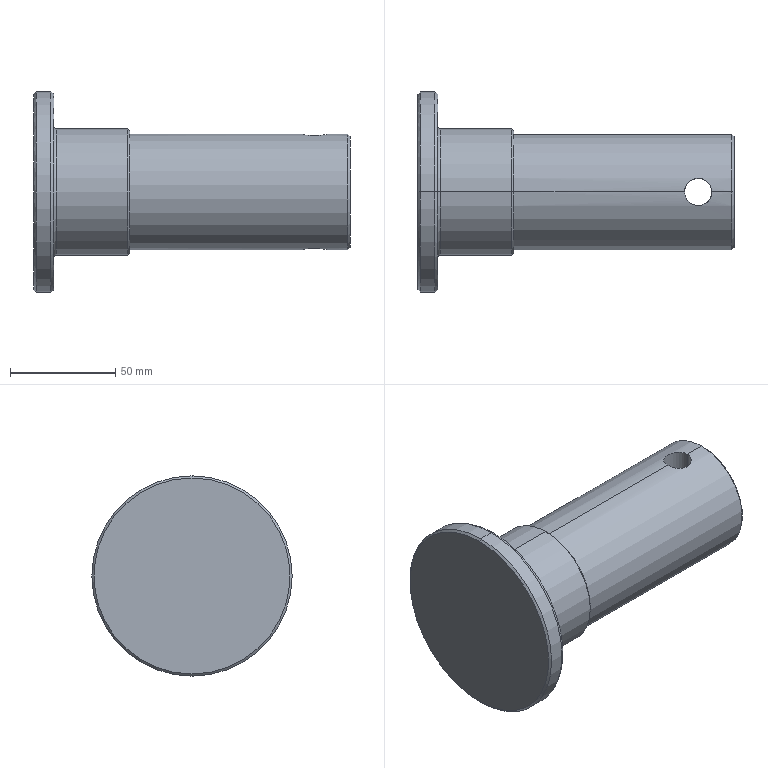Part | SolidWorks | features Chamfer 1, Fillet 1, ICE 1, Revolution 1 | 1 solid | 22 faces | box 150 x 95 x 95 mm | volume 409672 mm3 | cylinder 8 | cone 8 | plane 4 | torus 2 | commonest cylinder face diameters 13 x2 55 x2 60 x2 95 x2
STEP:
#1=CARTESIAN_POINT('',(126.5,0.,-27.5));
#2=VERTEX_POINT('',#1);
#3=CARTESIAN_POINT('',(139.5,0.,-27.5));
#4=VERTEX_POINT('',#3);
#5=CARTESIAN_POINT('',(126.5,0.,-27.5));
#6=CARTESIAN_POINT('',(126.5,-0.425,-27.5));
#7=CARTESIAN_POINT('',(126.541,-0.8485,-27.49));
#8=CARTESIAN_POINT('',(126.709,-1.692,-27.451));
#9=CARTESIAN_POINT('',(126.834,-2.099,-27.423));
#10=CARTESIAN_POINT('',(127.077,-2.687,-27.369));
#11=CARTESIAN_POINT('',(127.168,-2.878,-27.35));
#12=CARTESIAN_POINT('',(127.369,-3.254,-27.307));
#13=CARTESIAN_POINT('',(127.48,-3.439,-27.285));
#14=CARTESIAN_POINT('',(127.834,-3.968,-27.215));
#15=CARTESIAN_POINT('',(128.102,-4.294,-27.164));
#16=CARTESIAN_POINT('',(128.701,-4.894,-27.063));
#17=CARTESIAN_POINT('',(129.034,-5.167,-27.011));
#18=CARTESIAN_POINT('',(129.736,-5.637,-26.917));
#19=CARTESIAN_POINT('',(130.109,-5.837,-26.874));
#20=CARTESIAN_POINT('',(130.702,-6.084,-26.819));
#21=CARTESIAN_POINT('',(130.904,-6.156,-26.802));
#22=CARTESIAN_POINT('',(131.311,-6.28,-26.773));
#23=CARTESIAN_POINT('',(131.722,-6.384,-26.749));
#24=CARTESIAN_POINT('',(132.143,-6.447,-26.734));
#25=CARTESIAN_POINT('',(132.567,-6.489,-26.723));
#26=CARTESIAN_POINT('',(132.783,-6.5,-26.721));
#27=CARTESIAN_POINT('',(133.426,-6.5,-26.721));
#28=CARTESIAN_POINT('',(133.849,-6.458,-26.731));
#29=CARTESIAN_POINT('',(134.684,-6.293,-26.771));
#30=CARTESIAN_POINT('',(135.098,-6.167,-26.8));
#31=CARTESIAN_POINT('',(135.883,-5.841,-26.873));
#32=CARTESIAN_POINT('',(136.256,-5.642,-26.916));
#33=CARTESIAN_POINT('',(136.787,-5.287,-26.987));
#34=CARTESIAN_POINT('',(136.96,-5.159,-27.012));
#35=CARTESIAN_POINT('',(137.288,-4.89,-27.062));
#36=CARTESIAN_POINT('',(137.444,-4.748,-27.087));
#37=CARTESIAN_POINT('',(137.892,-4.301,-27.163));
#38=CARTESIAN_POINT('',(138.163,-3.972,-27.214));
#39=CARTESIAN_POINT('',(138.638,-3.263,-27.308));
#40=CARTESIAN_POINT('',(138.838,-2.89,-27.351));
#41=CARTESIAN_POINT('',(139.082,-2.303,-27.404));
#42=CARTESIAN_POINT('',(139.154,-2.103,-27.42));
#43=CARTESIAN_POINT('',(139.279,-1.693,-27.449));
#44=CARTESIAN_POINT('',(139.332,-1.484,-27.461));
#45=CARTESIAN_POINT('',(139.458,-0.8559,-27.49));
#46=CARTESIAN_POINT('',(139.5,-0.431,-27.5));
#47=CARTESIAN_POINT('',(139.5,0.,-27.5));
#48=B_SPLINE_CURVE_WITH_KNOTS('',3,(#5,#6,#7,#8,#9,#10,#11,#12,#13,#14,#15,#16,#17,#18,#19,#20,#21,#22,#23,#24,#25,#26,#27,#28,#29,#30,#31,#32,#33,#34,#35,#36,#37,#38,#39,#40,#41,#42,#43,#44,#45,#46,#47),.UNSPECIFIED.,.F.,.F.,(4,2,2,2,2,2,2,2,2,1,2,2,2,2,2,2,2,2,2,2,2,4),(0.02039,0.02167,0.02294,0.02358,0.02422,0.02549,0.02677,0.02804,0.02868,0.02931,0.02995,0.03059,0.03186,0.03314,0.03441,0.03505,0.03569,0.03696,0.03823,0.03887,0.03951,0.04078),.UNSPECIFIED.);
#49=EDGE_CURVE('',#2,#4,#48,.T.);
#50=ORIENTED_EDGE('',*,*,#49,.F.);
#51=CARTESIAN_POINT('',(126.5,0.,27.5));
#52=VERTEX_POINT('',#51);
#53=CARTESIAN_POINT('',(126.5,0.,-47.5));
#54=DIRECTION('',(0.,0.,1.));
#55=VECTOR('',#54,1000.);
#56=LINE('',#53,#55);
#57=EDGE_CURVE('',#2,#52,#56,.T.);
#58=ORIENTED_EDGE('',*,*,#57,.T.);
#59=CARTESIAN_POINT('',(139.5,0.,27.5));
#60=VERTEX_POINT('',#59);
#61=CARTESIAN_POINT('',(139.5,0.,27.5));
#62=CARTESIAN_POINT('',(139.5,-0.4311,27.5));
#63=CARTESIAN_POINT('',(139.458,-0.8547,27.49));
#64=CARTESIAN_POINT('',(139.333,-1.479,27.461));
#65=CARTESIAN_POINT('',(139.281,-1.686,27.449));
#66=CARTESIAN_POINT('',(139.157,-2.095,27.421));
#67=CARTESIAN_POINT('',(139.084,-2.298,27.405));
#68=CARTESIAN_POINT('',(138.839,-2.888,27.351));
#69=CARTESIAN_POINT('',(138.639,-3.261,27.308));
#70=CARTESIAN_POINT('',(138.285,-3.79,27.238));
#71=CARTESIAN_POINT('',(138.157,-3.962,27.214));
#72=CARTESIAN_POINT('',(137.887,-4.291,27.164));
#73=CARTESIAN_POINT('',(137.744,-4.448,27.138));
#74=CARTESIAN_POINT('',(137.296,-4.896,27.062));
#75=CARTESIAN_POINT('',(136.97,-5.165,27.012));
#76=CARTESIAN_POINT('',(136.26,-5.64,26.917));
#77=CARTESIAN_POINT('',(135.884,-5.841,26.873));
#78=CARTESIAN_POINT('',(135.298,-6.084,26.819));
#79=CARTESIAN_POINT('',(135.098,-6.156,26.802));
#80=CARTESIAN_POINT('',(134.69,-6.28,26.773));
#81=CARTESIAN_POINT('',(134.481,-6.333,26.761));
#82=CARTESIAN_POINT('',(133.851,-6.458,26.731));
#83=CARTESIAN_POINT('',(133.428,-6.5,26.721));
#84=CARTESIAN_POINT('',(132.577,-6.5,26.721));
#85=CARTESIAN_POINT('',(132.145,-6.458,26.731));
#86=CARTESIAN_POINT('',(131.31,-6.291,26.771));
#87=CARTESIAN_POINT('',(130.904,-6.167,26.8));
#88=CARTESIAN_POINT('',(130.312,-5.922,26.855));
#89=CARTESIAN_POINT('',(130.117,-5.83,26.875));
#90=CARTESIAN_POINT('',(129.743,-5.629,26.918));
#91=CARTESIAN_POINT('',(129.561,-5.52,26.941));
#92=CARTESIAN_POINT('',(129.21,-5.285,26.988));
#93=CARTESIAN_POINT('',(129.04,-5.159,27.012));
#94=CARTESIAN_POINT('',(128.712,-4.89,27.062));
#95=CARTESIAN_POINT('',(128.554,-4.746,27.088));
#96=CARTESIAN_POINT('',(128.102,-4.294,27.164));
#97=CARTESIAN_POINT('',(127.834,-3.967,27.215));
#98=CARTESIAN_POINT('',(127.363,-3.265,27.308));
#99=CARTESIAN_POINT('',(127.159,-2.884,27.351));
#100=CARTESIAN_POINT('',(126.833,-2.099,27.423));
#101=CARTESIAN_POINT('',(126.71,-1.693,27.451));
#102=CARTESIAN_POINT('',(126.584,-1.066,27.48));
#103=CARTESIAN_POINT('',(126.553,-0.8521,27.488));
#104=CARTESIAN_POINT('',(126.51,-0.4255,27.498));
#105=CARTESIAN_POINT('',(126.5,-0.2125,27.5));
#106=CARTESIAN_POINT('',(126.5,0.,27.5));
#107=B_SPLINE_CURVE_WITH_KNOTS('',3,(#61,#62,#63,#64,#65,#66,#67,#68,#69,#70,#71,#72,#73,#74,#75,#76,#77,#78,#79,#80,#81,#82,#83,#84,#85,#86,#87,#88,#89,#90,#91,#92,#93,#94,#95,#96,#97,#98,#99,#100,#101,#102,#103,#104,#105,#106),.UNSPECIFIED.,.F.,.F.,(4,2,2,2,2,2,2,2,2,2,2,2,2,2,2,2,2,2,2,2,2,2,4),(0.,0.001275,0.001912,0.002549,0.003824,0.004461,0.005099,0.006373,0.007648,0.008285,0.008923,0.0102,0.01147,0.01275,0.01338,0.01402,0.01466,0.0153,0.01657,0.01785,0.01912,0.01976,0.02039),.UNSPECIFIED.);
#108=EDGE_CURVE('',#60,#52,#107,.T.);
#109=ORIENTED_EDGE('',*,*,#108,.F.);
#110=CARTESIAN_POINT('',(139.5,0.,-47.5));
#111=DIRECTION('',(0.,0.,1.));
#112=VECTOR('',#111,1000.);
#113=LINE('',#110,#112);
#114=EDGE_CURVE('',#4,#60,#113,.T.);
#115=ORIENTED_EDGE('',*,*,#114,.F.);
#116=EDGE_LOOP('',(#50,#58,#109,#115));
#117=FACE_OUTER_BOUND('',#116,.T.);
#118=CARTESIAN_POINT('',(133.,0.,-47.5));
#119=DIRECTION('',(0.,0.,1.));
#120=DIRECTION('',(1.,0.,0.));
#121=AXIS2_PLACEMENT_3D('',#118,#119,#120);
#122=CYLINDRICAL_SURFACE('',#121,6.5);
#123=ADVANCED_FACE('',(#117),#122,.F.);
#124=CARTESIAN_POINT('',(150.,0.,-26.5));
#125=VERTEX_POINT('',#124);
#126=CARTESIAN_POINT('',(150.,0.,26.5));
#127=VERTEX_POINT('',#126);
#128=CARTESIAN_POINT('',(150.,0.,0.));
#129=DIRECTION('',(1.,0.,0.));
#130=DIRECTION('',(0.,0.,1.));
#131=AXIS2_PLACEMENT_3D('',#128,#129,#130);
#132=CIRCLE('',#131,26.5);
#133=EDGE_CURVE('',#125,#127,#132,.T.);
#134=ORIENTED_EDGE('',*,*,#133,.F.);
#135=CARTESIAN_POINT('',(149.,0.,-27.5));
#136=VERTEX_POINT('',#135);
#137=CARTESIAN_POINT('',(149.,0.,-27.5));
#138=DIRECTION('',(-0.7071,0.,-0.7071));
#139=VECTOR('',#138,1000.);
#140=LINE('',#137,#139);
#141=EDGE_CURVE('',#125,#136,#140,.T.);
#142=ORIENTED_EDGE('',*,*,#141,.T.);
#143=CARTESIAN_POINT('',(149.,0.,27.5));
#144=VERTEX_POINT('',#143);
#145=CARTESIAN_POINT('',(149.,0.,0.));
#146=DIRECTION('',(-1.,0.,0.));
#147=DIRECTION('',(0.,0.,1.));
#148=AXIS2_PLACEMENT_3D('',#145,#146,#147);
#149=CIRCLE('',#148,27.5);
#150=EDGE_CURVE('',#144,#136,#149,.T.);
#151=ORIENTED_EDGE('',*,*,#150,.F.);
#152=CARTESIAN_POINT('',(149.,0.,27.5));
#153=DIRECTION('',(-0.7071,0.,0.7071));
#154=VECTOR('',#153,1000.);
#155=LINE('',#152,#154);
#156=EDGE_CURVE('',#127,#144,#155,.T.);
#157=ORIENTED_EDGE('',*,*,#156,.F.);
#158=EDGE_LOOP('',(#134,#142,#151,#157));
#159=FACE_OUTER_BOUND('',#158,.T.);
#160=CARTESIAN_POINT('',(149.,0.,0.));
#161=DIRECTION('',(-1.,0.,0.));
#162=DIRECTION('',(0.,0.,1.));
#163=AXIS2_PLACEMENT_3D('',#160,#161,#162);
#164=CONICAL_SURFACE('',#163,27.5,0.7854);
#165=ADVANCED_FACE('',(#159),#164,.T.);
#166=CARTESIAN_POINT('',(45.5,0.,-29.));
#167=VERTEX_POINT('',#166);
#168=CARTESIAN_POINT('',(45.5,0.,29.));
#169=VERTEX_POINT('',#168);
#170=CARTESIAN_POINT('',(45.5,0.,0.));
#171=DIRECTION('',(1.,0.,0.));
#172=DIRECTION('',(0.,0.,1.));
#173=AXIS2_PLACEMENT_3D('',#170,#171,#172);
#174=CIRCLE('',#173,29.);
#175=EDGE_CURVE('',#167,#169,#174,.T.);
#176=ORIENTED_EDGE('',*,*,#175,.F.);
#177=CARTESIAN_POINT('',(44.5,0.,-30.));
#178=VERTEX_POINT('',#177);
#179=CARTESIAN_POINT('',(44.5,0.,-30.));
#180=DIRECTION('',(-0.7071,0.,-0.7071));
#181=VECTOR('',#180,1000.);
#182=LINE('',#179,#181);
#183=EDGE_CURVE('',#167,#178,#182,.T.);
#184=ORIENTED_EDGE('',*,*,#183,.T.);
#185=CARTESIAN_POINT('',(44.5,0.,30.));
#186=VERTEX_POINT('',#185);
#187=CARTESIAN_POINT('',(44.5,0.,0.));
#188=DIRECTION('',(-1.,0.,0.));
#189=DIRECTION('',(0.,0.,1.));
#190=AXIS2_PLACEMENT_3D('',#187,#188,#189);
#191=CIRCLE('',#190,30.);
#192=EDGE_CURVE('',#186,#178,#191,.T.);
#193=ORIENTED_EDGE('',*,*,#192,.F.);
#194=CARTESIAN_POINT('',(44.5,0.,30.));
#195=DIRECTION('',(-0.7071,0.,0.7071));
#196=VECTOR('',#195,1000.);
#197=LINE('',#194,#196);
#198=EDGE_CURVE('',#169,#186,#197,.T.);
#199=ORIENTED_EDGE('',*,*,#198,.F.);
#200=EDGE_LOOP('',(#176,#184,#193,#199));
#201=FACE_OUTER_BOUND('',#200,.T.);
#202=CARTESIAN_POINT('',(44.5,0.,0.));
#203=DIRECTION('',(-1.,0.,0.));
#204=DIRECTION('',(0.,0.,1.));
#205=AXIS2_PLACEMENT_3D('',#202,#203,#204);
#206=CONICAL_SURFACE('',#205,30.,0.7854);
#207=ADVANCED_FACE('',(#201),#206,.T.);
#208=CARTESIAN_POINT('',(0.,0.,46.5));
#209=VERTEX_POINT('',#208);
#210=CARTESIAN_POINT('',(0.,0.,-46.5));
#211=VERTEX_POINT('',#210);
#212=CARTESIAN_POINT('',(0.,0.,0.));
#213=DIRECTION('',(-1.,0.,0.));
#214=DIRECTION('',(0.,0.,-1.));
#215=AXIS2_PLACEMENT_3D('',#212,#213,#214);
#216=CIRCLE('',#215,46.5);
#217=EDGE_CURVE('',#209,#211,#216,.T.);
#218=ORIENTED_EDGE('',*,*,#217,.F.);
#219=CARTESIAN_POINT('',(1.,0.,47.5));
#220=VERTEX_POINT('',#219);
#221=CARTESIAN_POINT('',(0.,0.,46.5));
#222=DIRECTION('',(0.7071,0.,0.7071));
#223=VECTOR('',#222,1000.);
#224=LINE('',#221,#223);
#225=EDGE_CURVE('',#209,#220,#224,.T.);
#226=ORIENTED_EDGE('',*,*,#225,.T.);
#227=CARTESIAN_POINT('',(1.,0.,-47.5));
#228=VERTEX_POINT('',#227);
#229=CARTESIAN_POINT('',(1.,0.,0.));
#230=DIRECTION('',(1.,0.,0.));
#231=DIRECTION('',(0.,0.,-1.));
#232=AXIS2_PLACEMENT_3D('',#229,#230,#231);
#233=CIRCLE('',#232,47.5);
#234=EDGE_CURVE('',#228,#220,#233,.T.);
#235=ORIENTED_EDGE('',*,*,#234,.F.);
#236=CARTESIAN_POINT('',(0.,0.,-46.5));
#237=DIRECTION('',(0.7071,0.,-0.7071));
#238=VECTOR('',#237,1000.);
#239=LINE('',#236,#238);
#240=EDGE_CURVE('',#211,#228,#239,.T.);
#241=ORIENTED_EDGE('',*,*,#240,.F.);
#242=EDGE_LOOP('',(#218,#226,#235,#241));
#243=FACE_OUTER_BOUND('',#242,.T.);
#244=CARTESIAN_POINT('',(0.,0.,0.));
#245=DIRECTION('',(1.,0.,0.));
#246=DIRECTION('',(0.,0.,-1.));
#247=AXIS2_PLACEMENT_3D('',#244,#245,#246);
#248=CONICAL_SURFACE('',#247,46.5,0.7854);
#249=ADVANCED_FACE('',(#243),#248,.T.);
#250=CARTESIAN_POINT('',(9.5,0.,-31.));
#251=VERTEX_POINT('',#250);
#252=CARTESIAN_POINT('',(9.5,0.,31.));
#253=VERTEX_POINT('',#252);
#254=CARTESIAN_POINT('',(9.5,0.,0.));
#255=DIRECTION('',(-1.,0.,0.));
#256=DIRECTION('',(0.,0.,1.));
#257=AXIS2_PLACEMENT_3D('',#254,#255,#256);
#258=CIRCLE('',#257,31.);
#259=EDGE_CURVE('',#251,#253,#258,.T.);
#260=ORIENTED_EDGE('',*,*,#259,.F.);
#261=CARTESIAN_POINT('',(10.5,0.,-30.));
#262=VERTEX_POINT('',#261);
#263=CARTESIAN_POINT('',(10.5,0.,-31.));
#264=DIRECTION('',(0.,1.,0.));
#265=DIRECTION('',(0.,0.,1.));
#266=AXIS2_PLACEMENT_3D('',#263,#264,#265);
#267=CIRCLE('',#266,1.);
#268=EDGE_CURVE('',#251,#262,#267,.T.);
#269=ORIENTED_EDGE('',*,*,#268,.T.);
#270=CARTESIAN_POINT('',(10.5,0.,30.));
#271=VERTEX_POINT('',#270);
#272=CARTESIAN_POINT('',(10.5,0.,0.));
#273=DIRECTION('',(1.,0.,0.));
#274=DIRECTION('',(0.,0.,1.));
#275=AXIS2_PLACEMENT_3D('',#272,#273,#274);
#276=CIRCLE('',#275,30.);
#277=EDGE_CURVE('',#271,#262,#276,.T.);
#278=ORIENTED_EDGE('',*,*,#277,.F.);
#279=CARTESIAN_POINT('',(10.5,0.,31.));
#280=DIRECTION('',(0.,-1.,0.));
#281=DIRECTION('',(0.,0.,-1.));
#282=AXIS2_PLACEMENT_3D('',#279,#280,#281);
#283=CIRCLE('',#282,1.);
#284=EDGE_CURVE('',#253,#271,#283,.T.);
#285=ORIENTED_EDGE('',*,*,#284,.F.);
#286=EDGE_LOOP('',(#260,#269,#278,#285));
#287=FACE_OUTER_BOUND('',#286,.T.);
#288=CARTESIAN_POINT('',(10.5,0.,0.));
#289=DIRECTION('',(-1.,0.,0.));
#290=DIRECTION('',(0.,0.,1.));
#291=AXIS2_PLACEMENT_3D('',#288,#289,#290);
#292=TOROIDAL_SURFACE('',#291,31.,1.);
#293=ADVANCED_FACE('',(#287),#292,.F.);
#294=ORIENTED_EDGE('',*,*,#150,.T.);
#295=CARTESIAN_POINT('',(0.,0.,-27.5));
#296=DIRECTION('',(-1.,0.,0.));
#297=VECTOR('',#296,1000.);
#298=LINE('',#295,#297);
#299=EDGE_CURVE('',#136,#4,#298,.T.);
#300=ORIENTED_EDGE('',*,*,#299,.T.);
#301=CARTESIAN_POINT('',(139.5,0.,-27.5));
#302=CARTESIAN_POINT('',(139.5,0.4311,-27.5));
#303=CARTESIAN_POINT('',(139.458,0.8547,-27.49));
#304=CARTESIAN_POINT('',(139.333,1.479,-27.461));
#305=CARTESIAN_POINT('',(139.281,1.686,-27.449));
#306=CARTESIAN_POINT('',(139.157,2.095,-27.421));
#307=CARTESIAN_POINT('',(139.084,2.298,-27.405));
#308=CARTESIAN_POINT('',(138.839,2.888,-27.351));
#309=CARTESIAN_POINT('',(138.639,3.261,-27.308));
#310=CARTESIAN_POINT('',(138.285,3.79,-27.238));
#311=CARTESIAN_POINT('',(138.157,3.962,-27.214));
#312=CARTESIAN_POINT('',(137.887,4.291,-27.164));
#313=CARTESIAN_POINT('',(137.744,4.448,-27.138));
#314=CARTESIAN_POINT('',(137.296,4.896,-27.062));
#315=CARTESIAN_POINT('',(136.97,5.165,-27.012));
#316=CARTESIAN_POINT('',(136.26,5.64,-26.917));
#317=CARTESIAN_POINT('',(135.884,5.841,-26.873));
#318=CARTESIAN_POINT('',(135.298,6.084,-26.819));
#319=CARTESIAN_POINT('',(135.098,6.156,-26.802));
#320=CARTESIAN_POINT('',(134.69,6.28,-26.773));
#321=CARTESIAN_POINT('',(134.481,6.333,-26.761));
#322=CARTESIAN_POINT('',(133.851,6.458,-26.731));
#323=CARTESIAN_POINT('',(133.428,6.5,-26.721));
#324=CARTESIAN_POINT('',(132.577,6.5,-26.721));
#325=CARTESIAN_POINT('',(132.145,6.458,-26.731));
#326=CARTESIAN_POINT('',(131.31,6.291,-26.771));
#327=CARTESIAN_POINT('',(130.904,6.167,-26.8));
#328=CARTESIAN_POINT('',(130.312,5.922,-26.855));
#329=CARTESIAN_POINT('',(130.117,5.83,-26.875));
#330=CARTESIAN_POINT('',(129.743,5.629,-26.918));
#331=CARTESIAN_POINT('',(129.561,5.52,-26.941));
#332=CARTESIAN_POINT('',(129.21,5.285,-26.988));
#333=CARTESIAN_POINT('',(129.04,5.159,-27.012));
#334=CARTESIAN_POINT('',(128.712,4.89,-27.062));
#335=CARTESIAN_POINT('',(128.554,4.746,-27.088));
#336=CARTESIAN_POINT('',(128.102,4.294,-27.164));
#337=CARTESIAN_POINT('',(127.834,3.967,-27.215));
#338=CARTESIAN_POINT('',(127.363,3.265,-27.308));
#339=CARTESIAN_POINT('',(127.159,2.884,-27.351));
#340=CARTESIAN_POINT('',(126.833,2.099,-27.423));
#341=CARTESIAN_POINT('',(126.71,1.693,-27.451));
#342=CARTESIAN_POINT('',(126.584,1.066,-27.48));
#343=CARTESIAN_POINT('',(126.553,0.8521,-27.488));
#344=CARTESIAN_POINT('',(126.51,0.4255,-27.498));
#345=CARTESIAN_POINT('',(126.5,0.2125,-27.5));
#346=CARTESIAN_POINT('',(126.5,0.,-27.5));
#347=B_SPLINE_CURVE_WITH_KNOTS('',3,(#301,#302,#303,#304,#305,#306,#307,#308,#309,#310,#311,#312,#313,#314,#315,#316,#317,#318,#319,#320,#321,#322,#323,#324,#325,#326,#327,#328,#329,#330,#331,#332,#333,#334,#335,#336,#337,#338,#339,#340,#341,#342,#343,#344,#345,#346),.UNSPECIFIED.,.F.,.F.,(4,2,2,2,2,2,2,2,2,2,2,2,2,2,2,2,2,2,2,2,2,2,4),(0.,0.001275,0.001912,0.002549,0.003824,0.004461,0.005099,0.006373,0.007648,0.008285,0.008923,0.0102,0.01147,0.01275,0.01338,0.01402,0.01466,0.0153,0.01657,0.01785,0.01912,0.01976,0.02039),.UNSPECIFIED.);
#348=EDGE_CURVE('',#4,#2,#347,.T.);
#349=ORIENTED_EDGE('',*,*,#348,.T.);
#350=CARTESIAN_POINT('',(45.5,0.,-27.5));
#351=VERTEX_POINT('',#350);
#352=CARTESIAN_POINT('',(0.,0.,-27.5));
#353=DIRECTION('',(-1.,0.,0.));
#354=VECTOR('',#353,1000.);
#355=LINE('',#352,#354);
#356=EDGE_CURVE('',#2,#351,#355,.T.);
#357=ORIENTED_EDGE('',*,*,#356,.T.);
#358=CARTESIAN_POINT('',(45.5,0.,27.5));
#359=VERTEX_POINT('',#358);
#360=CARTESIAN_POINT('',(45.5,0.,0.));
#361=DIRECTION('',(-1.,0.,0.));
#362=DIRECTION('',(0.,0.,1.));
#363=AXIS2_PLACEMENT_3D('',#360,#361,#362);
#364=CIRCLE('',#363,27.5);
#365=EDGE_CURVE('',#359,#351,#364,.T.);
#366=ORIENTED_EDGE('',*,*,#365,.F.);
#367=CARTESIAN_POINT('',(0.,0.,27.5));
#368=DIRECTION('',(-1.,0.,0.));
#369=VECTOR('',#368,1000.);
#370=LINE('',#367,#369);
#371=EDGE_CURVE('',#52,#359,#370,.T.);
#372=ORIENTED_EDGE('',*,*,#371,.F.);
#373=CARTESIAN_POINT('',(126.5,0.,27.5));
#374=CARTESIAN_POINT('',(126.5,0.425,27.5));
#375=CARTESIAN_POINT('',(126.541,0.8485,27.49));
#376=CARTESIAN_POINT('',(126.709,1.692,27.451));
#377=CARTESIAN_POINT('',(126.834,2.099,27.423));
#378=CARTESIAN_POINT('',(127.077,2.687,27.369));
#379=CARTESIAN_POINT('',(127.168,2.878,27.35));
#380=CARTESIAN_POINT('',(127.369,3.254,27.307));
#381=CARTESIAN_POINT('',(127.48,3.439,27.285));
#382=CARTESIAN_POINT('',(127.834,3.968,27.215));
#383=CARTESIAN_POINT('',(128.102,4.294,27.164));
#384=CARTESIAN_POINT('',(128.701,4.894,27.063));
#385=CARTESIAN_POINT('',(129.034,5.167,27.011));
#386=CARTESIAN_POINT('',(129.736,5.637,26.917));
#387=CARTESIAN_POINT('',(130.109,5.837,26.874));
#388=CARTESIAN_POINT('',(130.702,6.084,26.819));
#389=CARTESIAN_POINT('',(130.904,6.156,26.802));
#390=CARTESIAN_POINT('',(131.311,6.28,26.773));
#391=CARTESIAN_POINT('',(131.722,6.384,26.749));
#392=CARTESIAN_POINT('',(132.143,6.447,26.734));
#393=CARTESIAN_POINT('',(132.567,6.489,26.723));
#394=CARTESIAN_POINT('',(132.783,6.5,26.721));
#395=CARTESIAN_POINT('',(133.426,6.5,26.721));
#396=CARTESIAN_POINT('',(133.849,6.458,26.731));
#397=CARTESIAN_POINT('',(134.684,6.293,26.771));
#398=CARTESIAN_POINT('',(135.098,6.167,26.8));
#399=CARTESIAN_POINT('',(135.883,5.841,26.873));
#400=CARTESIAN_POINT('',(136.256,5.642,26.916));
#401=CARTESIAN_POINT('',(136.787,5.287,26.987));
#402=CARTESIAN_POINT('',(136.96,5.159,27.012));
#403=CARTESIAN_POINT('',(137.288,4.89,27.062));
#404=CARTESIAN_POINT('',(137.444,4.748,27.087));
#405=CARTESIAN_POINT('',(137.892,4.301,27.163));
#406=CARTESIAN_POINT('',(138.163,3.972,27.214));
#407=CARTESIAN_POINT('',(138.638,3.263,27.308));
#408=CARTESIAN_POINT('',(138.838,2.89,27.351));
#409=CARTESIAN_POINT('',(139.082,2.303,27.404));
#410=CARTESIAN_POINT('',(139.154,2.103,27.42));
#411=CARTESIAN_POINT('',(139.279,1.693,27.449));
#412=CARTESIAN_POINT('',(139.332,1.484,27.461));
#413=CARTESIAN_POINT('',(139.458,0.8559,27.49));
#414=CARTESIAN_POINT('',(139.5,0.431,27.5));
#415=CARTESIAN_POINT('',(139.5,0.,27.5));
#416=B_SPLINE_CURVE_WITH_KNOTS('',3,(#373,#374,#375,#376,#377,#378,#379,#380,#381,#382,#383,#384,#385,#386,#387,#388,#389,#390,#391,#392,#393,#394,#395,#396,#397,#398,#399,#400,#401,#402,#403,#404,#405,#406,#407,#408,#409,#410,#411,#412,#413,#414,#415),.UNSPECIFIED.,.F.,.F.,(4,2,2,2,2,2,2,2,2,1,2,2,2,2,2,2,2,2,2,2,2,4),(0.02039,0.02167,0.02294,0.02358,0.02422,0.02549,0.02677,0.02804,0.02868,0.02931,0.02995,0.03059,0.03186,0.03314,0.03441,0.03505,0.03569,0.03696,0.03823,0.03887,0.03951,0.04078),.UNSPECIFIED.);
#417=EDGE_CURVE('',#52,#60,#416,.T.);
#418=ORIENTED_EDGE('',*,*,#417,.T.);
#419=CARTESIAN_POINT('',(0.,0.,27.5));
#420=DIRECTION('',(-1.,0.,0.));
#421=VECTOR('',#420,1000.);
#422=LINE('',#419,#421);
#423=EDGE_CURVE('',#144,#60,#422,.T.);
#424=ORIENTED_EDGE('',*,*,#423,.F.);
#425=EDGE_LOOP('',(#294,#300,#349,#357,#366,#372,#418,#424));
#426=FACE_OUTER_BOUND('',#425,.T.);
#427=CARTESIAN_POINT('',(0.,0.,0.));
#428=DIRECTION('',(-1.,0.,0.));
#429=DIRECTION('',(0.,0.,1.));
#430=AXIS2_PLACEMENT_3D('',#427,#428,#429);
#431=CYLINDRICAL_SURFACE('',#430,27.5);
#432=ADVANCED_FACE('',(#426),#431,.T.);
#433=ORIENTED_EDGE('',*,*,#192,.T.);
#434=CARTESIAN_POINT('',(0.,0.,-30.));
#435=DIRECTION('',(-1.,0.,0.));
#436=VECTOR('',#435,1000.);
#437=LINE('',#434,#436);
#438=EDGE_CURVE('',#178,#262,#437,.T.);
#439=ORIENTED_EDGE('',*,*,#438,.T.);
#440=CARTESIAN_POINT('',(10.5,0.,0.));
#441=DIRECTION('',(1.,0.,0.));
#442=DIRECTION('',(0.,0.,1.));
#443=AXIS2_PLACEMENT_3D('',#440,#441,#442);
#444=CIRCLE('',#443,30.);
#445=EDGE_CURVE('',#262,#271,#444,.T.);
#446=ORIENTED_EDGE('',*,*,#445,.T.);
#447=CARTESIAN_POINT('',(0.,0.,30.));
#448=DIRECTION('',(-1.,0.,0.));
#449=VECTOR('',#448,1000.);
#450=LINE('',#447,#449);
#451=EDGE_CURVE('',#186,#271,#450,.T.);
#452=ORIENTED_EDGE('',*,*,#451,.F.);
#453=EDGE_LOOP('',(#433,#439,#446,#452));
#454=FACE_OUTER_BOUND('',#453,.T.);
#455=CARTESIAN_POINT('',(0.,0.,0.));
#456=DIRECTION('',(-1.,0.,0.));
#457=DIRECTION('',(0.,0.,1.));
#458=AXIS2_PLACEMENT_3D('',#455,#456,#457);
#459=CYLINDRICAL_SURFACE('',#458,30.);
#460=ADVANCED_FACE('',(#454),#459,.T.);
#461=CARTESIAN_POINT('',(9.5,0.,46.634));
#462=VERTEX_POINT('',#461);
#463=CARTESIAN_POINT('',(9.5,0.,-46.634));
#464=VERTEX_POINT('',#463);
#465=CARTESIAN_POINT('',(9.5,0.,0.));
#466=DIRECTION('',(-1.,0.,0.));
#467=DIRECTION('',(0.,0.,1.));
#468=AXIS2_PLACEMENT_3D('',#465,#466,#467);
#469=CIRCLE('',#468,46.634);
#470=EDGE_CURVE('',#462,#464,#469,.T.);
#471=ORIENTED_EDGE('',*,*,#470,.T.);
#472=CARTESIAN_POINT('',(8.,0.,-47.5));
#473=VERTEX_POINT('',#472);
#474=CARTESIAN_POINT('',(9.5,0.,-46.634));
#475=DIRECTION('',(-0.866,0.,-0.5));
#476=VECTOR('',#475,1000.);
#477=LINE('',#474,#476);
#478=EDGE_CURVE('',#464,#473,#477,.T.);
#479=ORIENTED_EDGE('',*,*,#478,.T.);
#480=CARTESIAN_POINT('',(8.,0.,47.5));
#481=VERTEX_POINT('',#480);
#482=CARTESIAN_POINT('',(8.,0.,0.));
#483=DIRECTION('',(-1.,0.,0.));
#484=DIRECTION('',(0.,0.,1.));
#485=AXIS2_PLACEMENT_3D('',#482,#483,#484);
#486=CIRCLE('',#485,47.5);
#487=EDGE_CURVE('',#481,#473,#486,.T.);
#488=ORIENTED_EDGE('',*,*,#487,.F.);
#489=CARTESIAN_POINT('',(9.5,0.,46.634));
#490=DIRECTION('',(-0.866,0.,0.5));
#491=VECTOR('',#490,1000.);
#492=LINE('',#489,#491);
#493=EDGE_CURVE('',#462,#481,#492,.T.);
#494=ORIENTED_EDGE('',*,*,#493,.F.);
#495=EDGE_LOOP('',(#471,#479,#488,#494));
#496=FACE_OUTER_BOUND('',#495,.T.);
#497=CARTESIAN_POINT('',(9.5,0.,0.));
#498=DIRECTION('',(-1.,0.,0.));
#499=DIRECTION('',(0.,0.,1.));
#500=AXIS2_PLACEMENT_3D('',#497,#498,#499);
#501=CONICAL_SURFACE('',#500,46.634,0.5236);
#502=ADVANCED_FACE('',(#496),#501,.T.);
#503=ORIENTED_EDGE('',*,*,#487,.T.);
#504=CARTESIAN_POINT('',(0.,0.,-47.5));
#505=DIRECTION('',(-1.,0.,0.));
#506=VECTOR('',#505,1000.);
#507=LINE('',#504,#506);
#508=EDGE_CURVE('',#473,#228,#507,.T.);
#509=ORIENTED_EDGE('',*,*,#508,.T.);
#510=ORIENTED_EDGE('',*,*,#234,.T.);
#511=CARTESIAN_POINT('',(0.,0.,47.5));
#512=DIRECTION('',(-1.,0.,0.));
#513=VECTOR('',#512,1000.);
#514=LINE('',#511,#513);
#515=EDGE_CURVE('',#481,#220,#514,.T.);
#516=ORIENTED_EDGE('',*,*,#515,.F.);
#517=EDGE_LOOP('',(#503,#509,#510,#516));
#518=FACE_OUTER_BOUND('',#517,.T.);
#519=CARTESIAN_POINT('',(0.,0.,0.));
#520=DIRECTION('',(-1.,0.,0.));
#521=DIRECTION('',(0.,0.,1.));
#522=AXIS2_PLACEMENT_3D('',#519,#520,#521);
#523=CYLINDRICAL_SURFACE('',#522,47.5);
#524=ADVANCED_FACE('',(#518),#523,.T.);
#525=CARTESIAN_POINT('',(0.,0.,0.));
#526=DIRECTION('',(-1.,0.,0.));
#527=DIRECTION('',(0.,0.,-1.));
#528=AXIS2_PLACEMENT_3D('',#525,#526,#527);
#529=CIRCLE('',#528,46.5);
#530=EDGE_CURVE('',#211,#209,#529,.T.);
#531=ORIENTED_EDGE('',*,*,#530,.T.);
#532=ORIENTED_EDGE('',*,*,#217,.T.);
#533=EDGE_LOOP('',(#531,#532));
#534=FACE_OUTER_BOUND('',#533,.T.);
#535=CARTESIAN_POINT('',(0.,0.,0.));
#536=DIRECTION('',(1.,0.,0.));
#537=DIRECTION('',(0.,0.,-1.));
#538=AXIS2_PLACEMENT_3D('',#535,#536,#537);
#539=PLANE('',#538);
#540=ADVANCED_FACE('',(#534),#539,.F.);
#541=ORIENTED_EDGE('',*,*,#508,.F.);
#542=CARTESIAN_POINT('',(8.,0.,0.));
#543=DIRECTION('',(-1.,0.,0.));
#544=DIRECTION('',(0.,0.,1.));
#545=AXIS2_PLACEMENT_3D('',#542,#543,#544);
#546=CIRCLE('',#545,47.5);
#547=EDGE_CURVE('',#473,#481,#546,.T.);
#548=ORIENTED_EDGE('',*,*,#547,.T.);
#549=ORIENTED_EDGE('',*,*,#515,.T.);
#550=CARTESIAN_POINT('',(1.,0.,0.));
#551=DIRECTION('',(1.,0.,0.));
#552=DIRECTION('',(0.,0.,-1.));
#553=AXIS2_PLACEMENT_3D('',#550,#551,#552);
#554=CIRCLE('',#553,47.5);
#555=EDGE_CURVE('',#220,#228,#554,.T.);
#556=ORIENTED_EDGE('',*,*,#555,.T.);
#557=EDGE_LOOP('',(#541,#548,#549,#556));
#558=FACE_OUTER_BOUND('',#557,.T.);
#559=CARTESIAN_POINT('',(0.,0.,0.));
#560=DIRECTION('',(-1.,0.,0.));
#561=DIRECTION('',(0.,0.,1.));
#562=AXIS2_PLACEMENT_3D('',#559,#560,#561);
#563=CYLINDRICAL_SURFACE('',#562,47.5);
#564=ADVANCED_FACE('',(#558),#563,.T.);
#565=ORIENTED_EDGE('',*,*,#478,.F.);
#566=CARTESIAN_POINT('',(9.5,0.,0.));
#567=DIRECTION('',(-1.,0.,0.));
#568=DIRECTION('',(0.,0.,1.));
#569=AXIS2_PLACEMENT_3D('',#566,#567,#568);
#570=CIRCLE('',#569,46.634);
#571=EDGE_CURVE('',#464,#462,#570,.T.);
#572=ORIENTED_EDGE('',*,*,#571,.T.);
#573=ORIENTED_EDGE('',*,*,#493,.T.);
#574=ORIENTED_EDGE('',*,*,#547,.F.);
#575=EDGE_LOOP('',(#565,#572,#573,#574));
#576=FACE_OUTER_BOUND('',#575,.T.);
#577=CARTESIAN_POINT('',(9.5,0.,0.));
#578=DIRECTION('',(-1.,0.,0.));
#579=DIRECTION('',(0.,0.,1.));
#580=AXIS2_PLACEMENT_3D('',#577,#578,#579);
#581=CONICAL_SURFACE('',#580,46.634,0.5236);
#582=ADVANCED_FACE('',(#576),#581,.T.);
#583=CARTESIAN_POINT('',(9.5,0.,0.));
#584=DIRECTION('',(-1.,0.,0.));
#585=DIRECTION('',(0.,0.,1.));
#586=AXIS2_PLACEMENT_3D('',#583,#584,#585);
#587=CIRCLE('',#586,31.);
#588=EDGE_CURVE('',#253,#251,#587,.T.);
#589=ORIENTED_EDGE('',*,*,#588,.T.);
#590=ORIENTED_EDGE('',*,*,#259,.T.);
#591=EDGE_LOOP('',(#589,#590));
#592=FACE_BOUND('',#591,.T.);
#593=ORIENTED_EDGE('',*,*,#470,.F.);
#594=ORIENTED_EDGE('',*,*,#571,.F.);
#595=EDGE_LOOP('',(#593,#594));
#596=FACE_OUTER_BOUND('',#595,.T.);
#597=CARTESIAN_POINT('',(9.5,46.634,0.));
#598=DIRECTION('',(-1.,0.,0.));
#599=DIRECTION('',(0.,0.,1.));
#600=AXIS2_PLACEMENT_3D('',#597,#598,#599);
#601=PLANE('',#600);
#602=ADVANCED_FACE('',(#592,#596),#601,.F.);
#603=ORIENTED_EDGE('',*,*,#438,.F.);
#604=CARTESIAN_POINT('',(44.5,0.,0.));
#605=DIRECTION('',(-1.,0.,0.));
#606=DIRECTION('',(0.,0.,1.));
#607=AXIS2_PLACEMENT_3D('',#604,#605,#606);
#608=CIRCLE('',#607,30.);
#609=EDGE_CURVE('',#178,#186,#608,.T.);
#610=ORIENTED_EDGE('',*,*,#609,.T.);
#611=ORIENTED_EDGE('',*,*,#451,.T.);
#612=ORIENTED_EDGE('',*,*,#277,.T.);
#613=EDGE_LOOP('',(#603,#610,#611,#612));
#614=FACE_OUTER_BOUND('',#613,.T.);
#615=CARTESIAN_POINT('',(0.,0.,0.));
#616=DIRECTION('',(-1.,0.,0.));
#617=DIRECTION('',(0.,0.,1.));
#618=AXIS2_PLACEMENT_3D('',#615,#616,#617);
#619=CYLINDRICAL_SURFACE('',#618,30.);
#620=ADVANCED_FACE('',(#614),#619,.T.);
#621=CARTESIAN_POINT('',(45.5,0.,0.));
#622=DIRECTION('',(1.,0.,0.));
#623=DIRECTION('',(0.,0.,1.));
#624=AXIS2_PLACEMENT_3D('',#621,#622,#623);
#625=CIRCLE('',#624,29.);
#626=EDGE_CURVE('',#169,#167,#625,.T.);
#627=ORIENTED_EDGE('',*,*,#626,.T.);
#628=ORIENTED_EDGE('',*,*,#175,.T.);
#629=EDGE_LOOP('',(#627,#628));
#630=FACE_OUTER_BOUND('',#629,.T.);
#631=ORIENTED_EDGE('',*,*,#365,.T.);
#632=CARTESIAN_POINT('',(45.5,0.,0.));
#633=DIRECTION('',(-1.,0.,0.));
#634=DIRECTION('',(0.,0.,1.));
#635=AXIS2_PLACEMENT_3D('',#632,#633,#634);
#636=CIRCLE('',#635,27.5);
#637=EDGE_CURVE('',#351,#359,#636,.T.);
#638=ORIENTED_EDGE('',*,*,#637,.T.);
#639=EDGE_LOOP('',(#631,#638));
#640=FACE_BOUND('',#639,.T.);
#641=CARTESIAN_POINT('',(45.5,30.,0.));
#642=DIRECTION('',(-1.,0.,0.));
#643=DIRECTION('',(0.,0.,1.));
#644=AXIS2_PLACEMENT_3D('',#641,#642,#643);
#645=PLANE('',#644);
#646=ADVANCED_FACE('',(#630,#640),#645,.F.);
#647=ORIENTED_EDGE('',*,*,#299,.F.);
#648=CARTESIAN_POINT('',(149.,0.,0.));
#649=DIRECTION('',(-1.,0.,0.));
#650=DIRECTION('',(0.,0.,1.));
#651=AXIS2_PLACEMENT_3D('',#648,#649,#650);
#652=CIRCLE('',#651,27.5);
#653=EDGE_CURVE('',#136,#144,#652,.T.);
#654=ORIENTED_EDGE('',*,*,#653,.T.);
#655=ORIENTED_EDGE('',*,*,#423,.T.);
#656=ORIENTED_EDGE('',*,*,#108,.T.);
#657=ORIENTED_EDGE('',*,*,#371,.T.);
#658=ORIENTED_EDGE('',*,*,#637,.F.);
#659=ORIENTED_EDGE('',*,*,#356,.F.);
#660=ORIENTED_EDGE('',*,*,#49,.T.);
#661=EDGE_LOOP('',(#647,#654,#655,#656,#657,#658,#659,#660));
#662=FACE_OUTER_BOUND('',#661,.T.);
#663=CARTESIAN_POINT('',(0.,0.,0.));
#664=DIRECTION('',(-1.,0.,0.));
#665=DIRECTION('',(0.,0.,1.));
#666=AXIS2_PLACEMENT_3D('',#663,#664,#665);
#667=CYLINDRICAL_SURFACE('',#666,27.5);
#668=ADVANCED_FACE('',(#662),#667,.T.);
#669=CARTESIAN_POINT('',(150.,0.,0.));
#670=DIRECTION('',(1.,0.,0.));
#671=DIRECTION('',(0.,0.,1.));
#672=AXIS2_PLACEMENT_3D('',#669,#670,#671);
#673=CIRCLE('',#672,26.5);
#674=EDGE_CURVE('',#127,#125,#673,.T.);
#675=ORIENTED_EDGE('',*,*,#674,.T.);
#676=ORIENTED_EDGE('',*,*,#133,.T.);
#677=EDGE_LOOP('',(#675,#676));
#678=FACE_OUTER_BOUND('',#677,.T.);
#679=CARTESIAN_POINT('',(150.,27.5,0.));
#680=DIRECTION('',(-1.,0.,0.));
#681=DIRECTION('',(0.,0.,1.));
#682=AXIS2_PLACEMENT_3D('',#679,#680,#681);
#683=PLANE('',#682);
#684=ADVANCED_FACE('',(#678),#683,.F.);
#685=ORIENTED_EDGE('',*,*,#268,.F.);
#686=ORIENTED_EDGE('',*,*,#588,.F.);
#687=ORIENTED_EDGE('',*,*,#284,.T.);
#688=ORIENTED_EDGE('',*,*,#445,.F.);
#689=EDGE_LOOP('',(#685,#686,#687,#688));
#690=FACE_OUTER_BOUND('',#689,.T.);
#691=CARTESIAN_POINT('',(10.5,0.,0.));
#692=DIRECTION('',(-1.,0.,0.));
#693=DIRECTION('',(0.,0.,1.));
#694=AXIS2_PLACEMENT_3D('',#691,#692,#693);
#695=TOROIDAL_SURFACE('',#694,31.,1.);
#696=ADVANCED_FACE('',(#690),#695,.F.);
#697=ORIENTED_EDGE('',*,*,#225,.F.);
#698=ORIENTED_EDGE('',*,*,#530,.F.);
#699=ORIENTED_EDGE('',*,*,#240,.T.);
#700=ORIENTED_EDGE('',*,*,#555,.F.);
#701=EDGE_LOOP('',(#697,#698,#699,#700));
#702=FACE_OUTER_BOUND('',#701,.T.);
#703=CARTESIAN_POINT('',(0.,0.,0.));
#704=DIRECTION('',(1.,0.,0.));
#705=DIRECTION('',(0.,0.,-1.));
#706=AXIS2_PLACEMENT_3D('',#703,#704,#705);
#707=CONICAL_SURFACE('',#706,46.5,0.7854);
#708=ADVANCED_FACE('',(#702),#707,.T.);
#709=ORIENTED_EDGE('',*,*,#183,.F.);
#710=ORIENTED_EDGE('',*,*,#626,.F.);
#711=ORIENTED_EDGE('',*,*,#198,.T.);
#712=ORIENTED_EDGE('',*,*,#609,.F.);
#713=EDGE_LOOP('',(#709,#710,#711,#712));
#714=FACE_OUTER_BOUND('',#713,.T.);
#715=CARTESIAN_POINT('',(44.5,0.,0.));
#716=DIRECTION('',(-1.,0.,0.));
#717=DIRECTION('',(0.,0.,1.));
#718=AXIS2_PLACEMENT_3D('',#715,#716,#717);
#719=CONICAL_SURFACE('',#718,30.,0.7854);
#720=ADVANCED_FACE('',(#714),#719,.T.);
#721=ORIENTED_EDGE('',*,*,#141,.F.);
#722=ORIENTED_EDGE('',*,*,#674,.F.);
#723=ORIENTED_EDGE('',*,*,#156,.T.);
#724=ORIENTED_EDGE('',*,*,#653,.F.);
#725=EDGE_LOOP('',(#721,#722,#723,#724));
#726=FACE_OUTER_BOUND('',#725,.T.);
#727=CARTESIAN_POINT('',(149.,0.,0.));
#728=DIRECTION('',(-1.,0.,0.));
#729=DIRECTION('',(0.,0.,1.));
#730=AXIS2_PLACEMENT_3D('',#727,#728,#729);
#731=CONICAL_SURFACE('',#730,27.5,0.7854);
#732=ADVANCED_FACE('',(#726),#731,.T.);
#733=ORIENTED_EDGE('',*,*,#57,.F.);
#734=ORIENTED_EDGE('',*,*,#348,.F.);
#735=ORIENTED_EDGE('',*,*,#114,.T.);
#736=ORIENTED_EDGE('',*,*,#417,.F.);
#737=EDGE_LOOP('',(#733,#734,#735,#736));
#738=FACE_OUTER_BOUND('',#737,.T.);
#739=CARTESIAN_POINT('',(133.,0.,-47.5));
#740=DIRECTION('',(0.,0.,1.));
#741=DIRECTION('',(1.,0.,0.));
#742=AXIS2_PLACEMENT_3D('',#739,#740,#741);
#743=CYLINDRICAL_SURFACE('',#742,6.5);
#744=ADVANCED_FACE('',(#738),#743,.F.);
#745=CLOSED_SHELL('',(#123,#165,#207,#249,#293,#432,#460,#502,#524,#540,#564,#582,#602,#620,#646,#668,#684,#696,#708,#720,#732,#744));
#746=MANIFOLD_SOLID_BREP('',#745);
#747=CARTESIAN_POINT('',(0.,0.,0.));
#748=DIRECTION('',(0.,0.,1.));
#749=DIRECTION('',(1.,0.,0.));
#750=AXIS2_PLACEMENT_3D('',#747,#748,#749);
#751=(LENGTH_UNIT()NAMED_UNIT(*)SI_UNIT(.MILLI.,.METRE.));
#752=UNCERTAINTY_MEASURE_WITH_UNIT(LENGTH_MEASURE(0.00001),#751,'','');
#753=(NAMED_UNIT(*)PLANE_ANGLE_UNIT()SI_UNIT($,.RADIAN.));
#754=(NAMED_UNIT(*)SI_UNIT($,.STERADIAN.)SOLID_ANGLE_UNIT());
#755=(GEOMETRIC_REPRESENTATION_CONTEXT(3)GLOBAL_UNCERTAINTY_ASSIGNED_CONTEXT((#752))GLOBAL_UNIT_ASSIGNED_CONTEXT((#751,#753,#754))REPRESENTATION_CONTEXT('',''));
#756=ADVANCED_BREP_SHAPE_REPRESENTATION('',(#746,#750),#755);